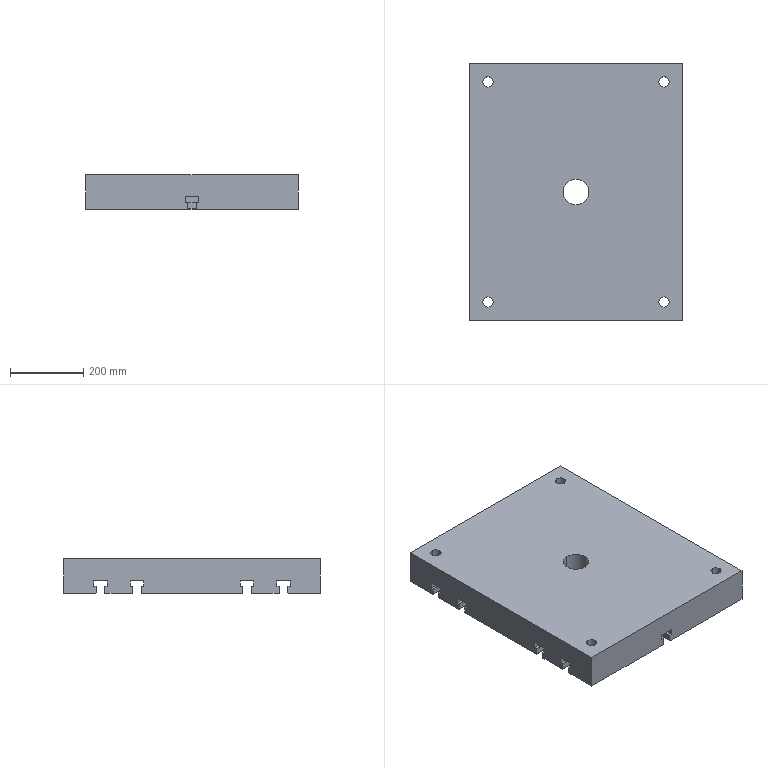Part | 1 solid | 128 faces | box 580 x 700 x 95 mm | volume 35310141 mm3 | plane 118 | cylinder 10 | commonest cylinder face diameters 28 x8 70 x2